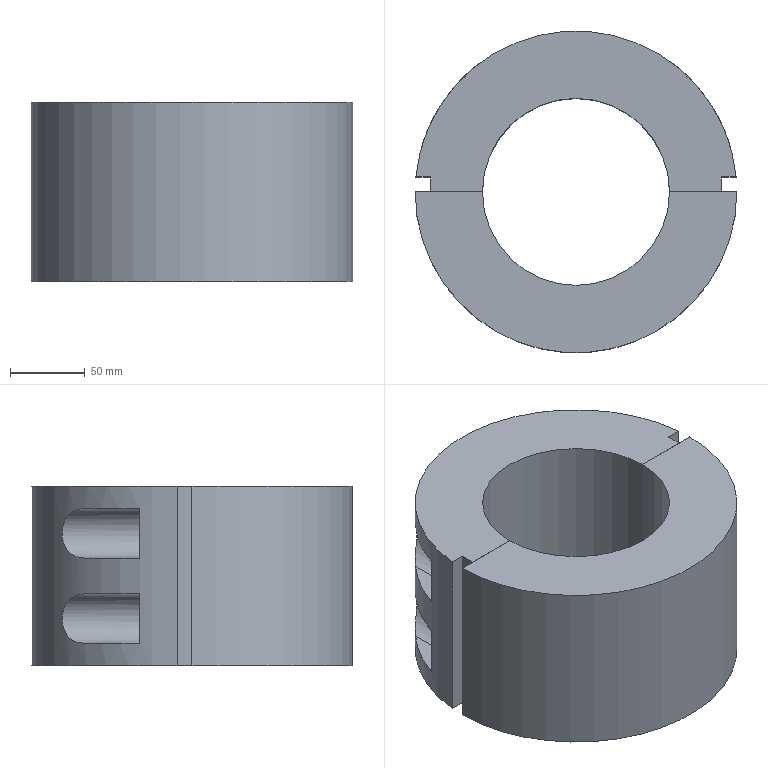NC program | NX | posted with a generic post | part box 215 x 215 x 120 mm
Whole program:
N10 G17 G21 G94 G90
(DRILLING_COPY_1 , TOOL : ZXZ)
N12 T02 M6
N14 G54
N16 G17 G0 G90 X-80. Y-28.5 S3500 M3
N18 G43 Z30. H2
N20 G94 G81 G98 Z-1. F250. R3.
N22 Y28.5
N24 X80.
N26 Y-28.5
N28 G80
N30 G0 X80. Y-28.5 Z30.
N32 M5
(DRILLING_COPY_COPY , TOOL : 17.5ZT)
N34 T04 M6
N36 G54
N38 G17 G0 G90 X-80. Y-28.5 S500 M3
N40 G43 Z30. H4
N42 G94 G83 G98 Z-40.258 F80. Q3. R3.
N44 Y28.5
N46 X80.
N48 Y-28.5
N50 G80
N52 G0 X80. Y-28.5 Z30.
N54 M5
N56 M2